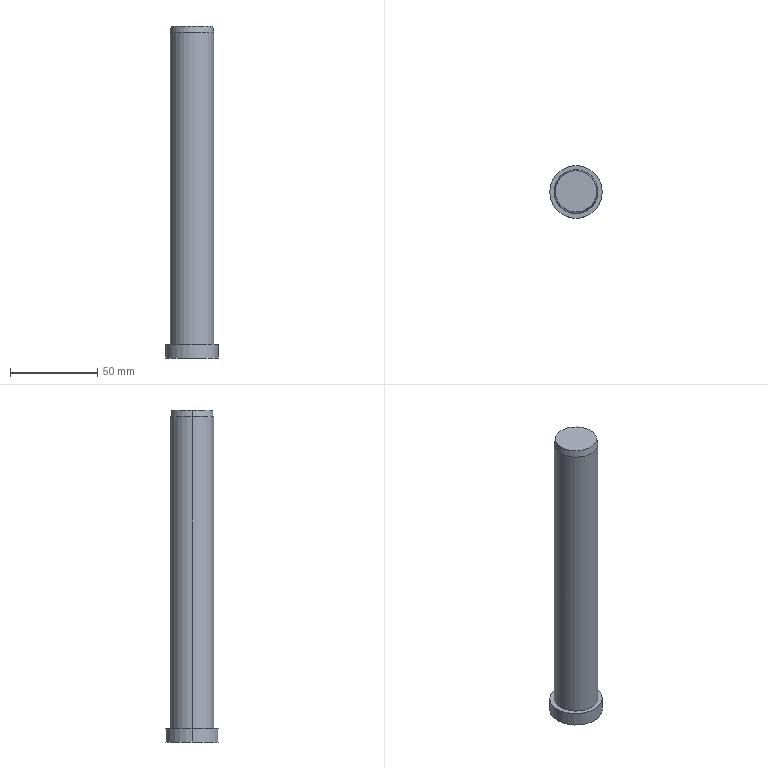Part | Creo | 1 solid | 15 faces | box 30 x 30 x 190 mm | volume 94190 mm3 | cylinder 8 | cone 4 | plane 3 | commonest cylinder face diameters 6.7 x2 25 x2 30 x2 7.98 x1 8 x1
STEP:
#1=CARTESIAN_POINT('',(0.,0.,0.));
#2=DIRECTION('',(0.,0.,1.));
#3=DIRECTION('',(1.,0.,0.));
#4=AXIS2_PLACEMENT_3D('',#1,#2,#3);
#5=CARTESIAN_POINT('',(-95.65,-141.,-276.5));
#6=VERTEX_POINT('',#5);
#7=CARTESIAN_POINT('',(-102.35,-141.,-276.5));
#8=VERTEX_POINT('',#7);
#9=CARTESIAN_POINT('',(-99.,-141.,-276.5));
#10=DIRECTION('',(0.,0.,-1.));
#11=DIRECTION('',(1.,0.,0.));
#12=AXIS2_PLACEMENT_3D('',#9,#10,#11);
#13=CIRCLE('',#12,3.35);
#14=EDGE_CURVE('',#6,#8,#13,.T.);
#15=ORIENTED_EDGE('',*,*,#14,.T.);
#16=CARTESIAN_POINT('',(-102.35,-141.,-295.5));
#17=VERTEX_POINT('',#16);
#18=CARTESIAN_POINT('',(-102.35,-141.,-295.5));
#19=DIRECTION('',(0.,0.,1.));
#20=VECTOR('',#19,19.);
#21=LINE('',#18,#20);
#22=EDGE_CURVE('',#17,#8,#21,.T.);
#23=ORIENTED_EDGE('',*,*,#22,.F.);
#24=CARTESIAN_POINT('',(-95.65,-141.,-295.5));
#25=VERTEX_POINT('',#24);
#26=CARTESIAN_POINT('',(-99.,-141.,-295.5));
#27=DIRECTION('',(0.,0.,1.));
#28=DIRECTION('',(-1.,0.,0.));
#29=AXIS2_PLACEMENT_3D('',#26,#27,#28);
#30=CIRCLE('',#29,3.35);
#31=EDGE_CURVE('',#17,#25,#30,.T.);
#32=ORIENTED_EDGE('',*,*,#31,.T.);
#33=CARTESIAN_POINT('',(-95.65,-141.,-295.5));
#34=DIRECTION('',(0.,0.,1.));
#35=VECTOR('',#34,19.);
#36=LINE('',#33,#35);
#37=EDGE_CURVE('',#25,#6,#36,.T.);
#38=ORIENTED_EDGE('',*,*,#37,.T.);
#39=EDGE_LOOP('',(#15,#23,#32,#38));
#40=FACE_OUTER_BOUND('',#39,.F.);
#41=CARTESIAN_POINT('',(-99.,-141.,-295.5));
#42=DIRECTION('',(0.,0.,1.));
#43=DIRECTION('',(1.,0.,0.));
#44=AXIS2_PLACEMENT_3D('',#41,#42,#43);
#45=CYLINDRICAL_SURFACE('',#44,3.35);
#46=ADVANCED_FACE('',(#40),#45,.F.);
#47=ORIENTED_EDGE('',*,*,#14,.F.);
#48=CARTESIAN_POINT('',(-99.,-141.,-274.487));
#49=VERTEX_POINT('',#48);
#50=CARTESIAN_POINT('',(-99.,-141.,-274.487));
#51=DIRECTION('',(0.8572,0.,-0.515));
#52=VECTOR('',#51,3.908);
#53=LINE('',#50,#52);
#54=EDGE_CURVE('',#49,#6,#53,.T.);
#55=ORIENTED_EDGE('',*,*,#54,.F.);
#56=CARTESIAN_POINT('',(-99.,-141.,-274.487));
#57=DIRECTION('',(-0.8572,0.,-0.515));
#58=VECTOR('',#57,3.908);
#59=LINE('',#56,#58);
#60=EDGE_CURVE('',#49,#8,#59,.T.);
#61=ORIENTED_EDGE('',*,*,#60,.T.);
#62=EDGE_LOOP('',(#47,#55,#61));
#63=FACE_OUTER_BOUND('',#62,.F.);
#64=CARTESIAN_POINT('',(-99.,-141.,-275.554));
#65=DIRECTION('',(0.,0.,-1.));
#66=DIRECTION('',(-1.,0.,0.));
#67=AXIS2_PLACEMENT_3D('',#64,#65,#66);
#68=CONICAL_SURFACE('',#67,1.775,59.);
#69=ADVANCED_FACE('',(#63),#68,.F.);
#70=CARTESIAN_POINT('',(-99.,-141.,-276.5));
#71=DIRECTION('',(0.,0.,-1.));
#72=DIRECTION('',(-1.,0.,0.));
#73=AXIS2_PLACEMENT_3D('',#70,#71,#72);
#74=CIRCLE('',#73,3.35);
#75=EDGE_CURVE('',#8,#6,#74,.T.);
#76=ORIENTED_EDGE('',*,*,#75,.F.);
#77=ORIENTED_EDGE('',*,*,#60,.F.);
#78=ORIENTED_EDGE('',*,*,#54,.T.);
#79=EDGE_LOOP('',(#76,#77,#78));
#80=FACE_OUTER_BOUND('',#79,.F.);
#81=CARTESIAN_POINT('',(-99.,-141.,-275.554));
#82=DIRECTION('',(0.,0.,-1.));
#83=DIRECTION('',(-1.,0.,0.));
#84=AXIS2_PLACEMENT_3D('',#81,#82,#83);
#85=CONICAL_SURFACE('',#84,1.775,59.);
#86=ADVANCED_FACE('',(#80),#85,.F.);
#87=ORIENTED_EDGE('',*,*,#75,.T.);
#88=ORIENTED_EDGE('',*,*,#37,.F.);
#89=CARTESIAN_POINT('',(-99.,-141.,-295.5));
#90=DIRECTION('',(0.,0.,1.));
#91=DIRECTION('',(1.,0.,0.));
#92=AXIS2_PLACEMENT_3D('',#89,#90,#91);
#93=CIRCLE('',#92,3.35);
#94=EDGE_CURVE('',#25,#17,#93,.T.);
#95=ORIENTED_EDGE('',*,*,#94,.T.);
#96=ORIENTED_EDGE('',*,*,#22,.T.);
#97=EDGE_LOOP('',(#87,#88,#95,#96));
#98=FACE_OUTER_BOUND('',#97,.F.);
#99=CARTESIAN_POINT('',(-99.,-141.,-295.5));
#100=DIRECTION('',(0.,0.,1.));
#101=DIRECTION('',(1.,0.,0.));
#102=AXIS2_PLACEMENT_3D('',#99,#100,#101);
#103=CYLINDRICAL_SURFACE('',#102,3.35);
#104=ADVANCED_FACE('',(#98),#103,.F.);
#105=CARTESIAN_POINT('',(-114.,-141.,-295.5));
#106=VERTEX_POINT('',#105);
#107=CARTESIAN_POINT('',(-84.,-141.,-295.5));
#108=VERTEX_POINT('',#107);
#109=CARTESIAN_POINT('',(-99.,-141.,-295.5));
#110=DIRECTION('',(0.,0.,-1.));
#111=DIRECTION('',(-1.,0.,0.));
#112=AXIS2_PLACEMENT_3D('',#109,#110,#111);
#113=CIRCLE('',#112,15.);
#114=EDGE_CURVE('',#106,#108,#113,.T.);
#115=ORIENTED_EDGE('',*,*,#114,.F.);
#116=CARTESIAN_POINT('',(-99.,-141.,-295.5));
#117=DIRECTION('',(0.,0.,-1.));
#118=DIRECTION('',(1.,0.,0.));
#119=AXIS2_PLACEMENT_3D('',#116,#117,#118);
#120=CIRCLE('',#119,15.);
#121=EDGE_CURVE('',#108,#106,#120,.T.);
#122=ORIENTED_EDGE('',*,*,#121,.F.);
#123=EDGE_LOOP('',(#115,#122));
#124=FACE_OUTER_BOUND('',#123,.F.);
#125=ORIENTED_EDGE('',*,*,#94,.F.);
#126=ORIENTED_EDGE('',*,*,#31,.F.);
#127=EDGE_LOOP('',(#125,#126));
#128=FACE_BOUND('',#127,.F.);
#129=CARTESIAN_POINT('',(-99.,-141.,-295.5));
#130=DIRECTION('',(0.,0.,-1.));
#131=DIRECTION('',(1.,0.,0.));
#132=AXIS2_PLACEMENT_3D('',#129,#130,#131);
#133=PLANE('',#132);
#134=ADVANCED_FACE('',(#124,#128),#133,.T.);
#135=CARTESIAN_POINT('',(-84.,-141.,-287.5));
#136=VERTEX_POINT('',#135);
#137=CARTESIAN_POINT('',(-114.,-141.,-287.5));
#138=VERTEX_POINT('',#137);
#139=CARTESIAN_POINT('',(-99.,-141.,-287.5));
#140=DIRECTION('',(0.,0.,1.));
#141=DIRECTION('',(1.,0.,0.));
#142=AXIS2_PLACEMENT_3D('',#139,#140,#141);
#143=CIRCLE('',#142,15.);
#144=EDGE_CURVE('',#136,#138,#143,.T.);
#145=ORIENTED_EDGE('',*,*,#144,.T.);
#146=CARTESIAN_POINT('',(-114.,-141.,-287.5));
#147=DIRECTION('',(0.,0.,-1.));
#148=VECTOR('',#147,8.);
#149=LINE('',#146,#148);
#150=EDGE_CURVE('',#138,#106,#149,.T.);
#151=ORIENTED_EDGE('',*,*,#150,.T.);
#152=ORIENTED_EDGE('',*,*,#114,.T.);
#153=CARTESIAN_POINT('',(-84.,-141.,-287.5));
#154=DIRECTION('',(0.,0.,-1.));
#155=VECTOR('',#154,8.);
#156=LINE('',#153,#155);
#157=EDGE_CURVE('',#136,#108,#156,.T.);
#158=ORIENTED_EDGE('',*,*,#157,.F.);
#159=EDGE_LOOP('',(#145,#151,#152,#158));
#160=FACE_OUTER_BOUND('',#159,.F.);
#161=CARTESIAN_POINT('',(-99.,-141.,-287.5));
#162=DIRECTION('',(0.,0.,-1.));
#163=DIRECTION('',(1.,0.,0.));
#164=AXIS2_PLACEMENT_3D('',#161,#162,#163);
#165=CYLINDRICAL_SURFACE('',#164,15.);
#166=ADVANCED_FACE('',(#160),#165,.T.);
#167=CARTESIAN_POINT('',(-99.,-141.,-287.5));
#168=DIRECTION('',(0.,0.,1.));
#169=DIRECTION('',(-1.,0.,0.));
#170=AXIS2_PLACEMENT_3D('',#167,#168,#169);
#171=CIRCLE('',#170,15.);
#172=EDGE_CURVE('',#138,#136,#171,.T.);
#173=ORIENTED_EDGE('',*,*,#172,.F.);
#174=ORIENTED_EDGE('',*,*,#144,.F.);
#175=EDGE_LOOP('',(#173,#174));
#176=FACE_OUTER_BOUND('',#175,.F.);
#177=CARTESIAN_POINT('',(-111.5,-141.,-287.5));
#178=VERTEX_POINT('',#177);
#179=CARTESIAN_POINT('',(-86.5,-141.,-287.5));
#180=VERTEX_POINT('',#179);
#181=CARTESIAN_POINT('',(-99.,-141.,-287.5));
#182=DIRECTION('',(0.,0.,-1.));
#183=DIRECTION('',(-1.,0.,0.));
#184=AXIS2_PLACEMENT_3D('',#181,#182,#183);
#185=CIRCLE('',#184,12.5);
#186=EDGE_CURVE('',#178,#180,#185,.T.);
#187=ORIENTED_EDGE('',*,*,#186,.F.);
#188=CARTESIAN_POINT('',(-99.,-141.,-287.5));
#189=DIRECTION('',(0.,0.,-1.));
#190=DIRECTION('',(1.,0.,0.));
#191=AXIS2_PLACEMENT_3D('',#188,#189,#190);
#192=CIRCLE('',#191,12.5);
#193=EDGE_CURVE('',#180,#178,#192,.T.);
#194=ORIENTED_EDGE('',*,*,#193,.F.);
#195=EDGE_LOOP('',(#187,#194));
#196=FACE_BOUND('',#195,.F.);
#197=CARTESIAN_POINT('',(-99.,-141.,-287.5));
#198=DIRECTION('',(0.,0.,-1.));
#199=DIRECTION('',(1.,0.,0.));
#200=AXIS2_PLACEMENT_3D('',#197,#198,#199);
#201=PLANE('',#200);
#202=ADVANCED_FACE('',(#176,#196),#201,.F.);
#203=CARTESIAN_POINT('',(-86.5,-141.,-109.5));
#204=VERTEX_POINT('',#203);
#205=CARTESIAN_POINT('',(-111.5,-141.,-109.5));
#206=VERTEX_POINT('',#205);
#207=CARTESIAN_POINT('',(-99.,-141.,-109.5));
#208=DIRECTION('',(0.,0.,1.));
#209=DIRECTION('',(1.,0.,0.));
#210=AXIS2_PLACEMENT_3D('',#207,#208,#209);
#211=CIRCLE('',#210,12.5);
#212=EDGE_CURVE('',#204,#206,#211,.T.);
#213=ORIENTED_EDGE('',*,*,#212,.T.);
#214=CARTESIAN_POINT('',(-111.5,-141.,-287.5));
#215=DIRECTION('',(0.,0.,1.));
#216=VECTOR('',#215,178.);
#217=LINE('',#214,#216);
#218=EDGE_CURVE('',#178,#206,#217,.T.);
#219=ORIENTED_EDGE('',*,*,#218,.F.);
#220=ORIENTED_EDGE('',*,*,#186,.T.);
#221=CARTESIAN_POINT('',(-86.5,-141.,-287.5));
#222=DIRECTION('',(0.,0.,1.));
#223=VECTOR('',#222,178.);
#224=LINE('',#221,#223);
#225=EDGE_CURVE('',#180,#204,#224,.T.);
#226=ORIENTED_EDGE('',*,*,#225,.T.);
#227=EDGE_LOOP('',(#213,#219,#220,#226));
#228=FACE_OUTER_BOUND('',#227,.F.);
#229=CARTESIAN_POINT('',(-99.,-141.,-287.5));
#230=DIRECTION('',(0.,0.,1.));
#231=DIRECTION('',(1.,0.,0.));
#232=AXIS2_PLACEMENT_3D('',#229,#230,#231);
#233=CYLINDRICAL_SURFACE('',#232,12.5);
#234=ADVANCED_FACE('',(#228),#233,.T.);
#235=ORIENTED_EDGE('',*,*,#212,.F.);
#236=CARTESIAN_POINT('',(-87.205,-141.,-105.5));
#237=VERTEX_POINT('',#236);
#238=CARTESIAN_POINT('',(-87.205,-141.,-105.5));
#239=DIRECTION('',(0.1736,0.,-0.9848));
#240=VECTOR('',#239,4.062);
#241=LINE('',#238,#240);
#242=EDGE_CURVE('',#237,#204,#241,.T.);
#243=ORIENTED_EDGE('',*,*,#242,.F.);
#244=CARTESIAN_POINT('',(-110.795,-141.,-105.5));
#245=VERTEX_POINT('',#244);
#246=CARTESIAN_POINT('',(-99.,-141.,-105.5));
#247=DIRECTION('',(0.,0.,1.));
#248=DIRECTION('',(1.,0.,0.));
#249=AXIS2_PLACEMENT_3D('',#246,#247,#248);
#250=CIRCLE('',#249,11.795);
#251=EDGE_CURVE('',#237,#245,#250,.T.);
#252=ORIENTED_EDGE('',*,*,#251,.T.);
#253=CARTESIAN_POINT('',(-110.795,-141.,-105.5));
#254=DIRECTION('',(-0.1736,0.,-0.9848));
#255=VECTOR('',#254,4.062);
#256=LINE('',#253,#255);
#257=EDGE_CURVE('',#245,#206,#256,.T.);
#258=ORIENTED_EDGE('',*,*,#257,.T.);
#259=EDGE_LOOP('',(#235,#243,#252,#258));
#260=FACE_OUTER_BOUND('',#259,.F.);
#261=CARTESIAN_POINT('',(-99.,-141.,-107.5));
#262=DIRECTION('',(0.,0.,-1.));
#263=DIRECTION('',(1.,0.,0.));
#264=AXIS2_PLACEMENT_3D('',#261,#262,#263);
#265=CONICAL_SURFACE('',#264,12.147,10.);
#266=ADVANCED_FACE('',(#260),#265,.T.);
#267=CARTESIAN_POINT('',(-99.,-141.,-109.5));
#268=DIRECTION('',(0.,0.,1.));
#269=DIRECTION('',(-1.,0.,0.));
#270=AXIS2_PLACEMENT_3D('',#267,#268,#269);
#271=CIRCLE('',#270,12.5);
#272=EDGE_CURVE('',#206,#204,#271,.T.);
#273=ORIENTED_EDGE('',*,*,#272,.F.);
#274=ORIENTED_EDGE('',*,*,#257,.F.);
#275=CARTESIAN_POINT('',(-99.,-141.,-105.5));
#276=DIRECTION('',(0.,0.,1.));
#277=DIRECTION('',(-1.,0.,0.));
#278=AXIS2_PLACEMENT_3D('',#275,#276,#277);
#279=CIRCLE('',#278,11.795);
#280=EDGE_CURVE('',#245,#237,#279,.T.);
#281=ORIENTED_EDGE('',*,*,#280,.T.);
#282=ORIENTED_EDGE('',*,*,#242,.T.);
#283=EDGE_LOOP('',(#273,#274,#281,#282));
#284=FACE_OUTER_BOUND('',#283,.F.);
#285=CARTESIAN_POINT('',(-99.,-141.,-107.5));
#286=DIRECTION('',(0.,0.,-1.));
#287=DIRECTION('',(1.,0.,0.));
#288=AXIS2_PLACEMENT_3D('',#285,#286,#287);
#289=CONICAL_SURFACE('',#288,12.147,10.);
#290=ADVANCED_FACE('',(#284),#289,.T.);
#291=ORIENTED_EDGE('',*,*,#272,.T.);
#292=ORIENTED_EDGE('',*,*,#225,.F.);
#293=ORIENTED_EDGE('',*,*,#193,.T.);
#294=ORIENTED_EDGE('',*,*,#218,.T.);
#295=EDGE_LOOP('',(#291,#292,#293,#294));
#296=FACE_OUTER_BOUND('',#295,.F.);
#297=CARTESIAN_POINT('',(-99.,-141.,-287.5));
#298=DIRECTION('',(0.,0.,1.));
#299=DIRECTION('',(1.,0.,0.));
#300=AXIS2_PLACEMENT_3D('',#297,#298,#299);
#301=CYLINDRICAL_SURFACE('',#300,12.5);
#302=ADVANCED_FACE('',(#296),#301,.T.);
#303=ORIENTED_EDGE('',*,*,#251,.F.);
#304=ORIENTED_EDGE('',*,*,#280,.F.);
#305=EDGE_LOOP('',(#303,#304));
#306=FACE_OUTER_BOUND('',#305,.F.);
#307=CARTESIAN_POINT('',(-99.,-141.,-105.5));
#308=DIRECTION('',(0.,0.,1.));
#309=DIRECTION('',(1.,0.,0.));
#310=AXIS2_PLACEMENT_3D('',#307,#308,#309);
#311=PLANE('',#310);
#312=ADVANCED_FACE('',(#306),#311,.T.);
#313=ORIENTED_EDGE('',*,*,#172,.T.);
#314=ORIENTED_EDGE('',*,*,#157,.T.);
#315=ORIENTED_EDGE('',*,*,#121,.T.);
#316=ORIENTED_EDGE('',*,*,#150,.F.);
#317=EDGE_LOOP('',(#313,#314,#315,#316));
#318=FACE_OUTER_BOUND('',#317,.F.);
#319=CARTESIAN_POINT('',(-99.,-141.,-287.5));
#320=DIRECTION('',(0.,0.,-1.));
#321=DIRECTION('',(1.,0.,0.));
#322=AXIS2_PLACEMENT_3D('',#319,#320,#321);
#323=CYLINDRICAL_SURFACE('',#322,15.);
#324=ADVANCED_FACE('',(#318),#323,.T.);
#325=CLOSED_SHELL('',(#46,#69,#86,#104,#134,#166,#202,#234,#266,#290,#302,#312,#324));
#326=CARTESIAN_POINT('',(-95.005,-141.,-295.5));
#327=VERTEX_POINT('',#326);
#328=CARTESIAN_POINT('',(-102.99,-141.,-295.5));
#329=VERTEX_POINT('',#328);
#330=CARTESIAN_POINT('',(-99.,-141.,-295.5));
#331=DIRECTION('',(0.,0.,1.));
#332=DIRECTION('',(1.,0.,0.));
#333=AXIS2_PLACEMENT_3D('',#330,#331,#332);
#334=CIRCLE('',#333,3.99);
#335=EDGE_CURVE('',#327,#329,#334,.T.);
#336=ORIENTED_EDGE('',*,*,#335,.F.);
#337=CARTESIAN_POINT('',(-95.01,-141.,-279.5));
#338=VERTEX_POINT('',#337);
#339=CARTESIAN_POINT('',(-95.005,-141.,-295.5));
#340=DIRECTION('',(0.,0.,1.));
#341=VECTOR('',#340,16.);
#342=LINE('',#339,#341);
#343=EDGE_CURVE('',#327,#338,#342,.T.);
#344=ORIENTED_EDGE('',*,*,#343,.T.);
#345=CARTESIAN_POINT('',(-102.99,-141.,-279.5));
#346=VERTEX_POINT('',#345);
#347=CARTESIAN_POINT('',(-99.,-141.,-279.5));
#348=DIRECTION('',(0.,0.,-1.));
#349=DIRECTION('',(-1.,0.,0.));
#350=AXIS2_PLACEMENT_3D('',#347,#348,#349);
#351=CIRCLE('',#350,3.99);
#352=EDGE_CURVE('',#346,#338,#351,.T.);
#353=ORIENTED_EDGE('',*,*,#352,.F.);
#354=CARTESIAN_POINT('',(-99.,-144.99,-279.5));
#355=VERTEX_POINT('',#354);
#356=CARTESIAN_POINT('',(-99.,-141.,-279.5));
#357=DIRECTION('',(0.,0.,-1.));
#358=DIRECTION('',(0.,-1.,0.));
#359=AXIS2_PLACEMENT_3D('',#356,#357,#358);
#360=CIRCLE('',#359,3.99);
#361=EDGE_CURVE('',#355,#346,#360,.T.);
#362=ORIENTED_EDGE('',*,*,#361,.F.);
#363=CARTESIAN_POINT('',(-99.,-144.995,-295.5));
#364=VERTEX_POINT('',#363);
#365=CARTESIAN_POINT('',(-99.,-144.995,-279.5));
#366=DIRECTION('',(0.,0.,-1.));
#367=VECTOR('',#366,16.);
#368=LINE('',#365,#367);
#369=EDGE_CURVE('',#355,#364,#368,.T.);
#370=ORIENTED_EDGE('',*,*,#369,.T.);
#371=CARTESIAN_POINT('',(-99.,-141.,-295.5));
#372=DIRECTION('',(0.,0.,1.));
#373=DIRECTION('',(-1.,-0.000002843,0.));
#374=AXIS2_PLACEMENT_3D('',#371,#372,#373);
#375=CIRCLE('',#374,3.99);
#376=EDGE_CURVE('',#329,#364,#375,.T.);
#377=ORIENTED_EDGE('',*,*,#376,.F.);
#378=EDGE_LOOP('',(#336,#344,#353,#362,#370,#377));
#379=FACE_OUTER_BOUND('',#378,.F.);
#380=CARTESIAN_POINT('',(-99.,-141.,-296.5));
#381=DIRECTION('',(0.,0.,1.));
#382=DIRECTION('',(1.,0.,0.));
#383=AXIS2_PLACEMENT_3D('',#380,#381,#382);
#384=CYLINDRICAL_SURFACE('',#383,4.);
#385=ADVANCED_FACE('',(#379),#384,.T.);
#386=ORIENTED_EDGE('',*,*,#335,.T.);
#387=ORIENTED_EDGE('',*,*,#376,.T.);
#388=ORIENTED_EDGE('',*,*,#369,.F.);
#389=ORIENTED_EDGE('',*,*,#361,.T.);
#390=ORIENTED_EDGE('',*,*,#352,.T.);
#391=ORIENTED_EDGE('',*,*,#343,.F.);
#392=EDGE_LOOP('',(#386,#387,#388,#389,#390,#391));
#393=FACE_OUTER_BOUND('',#392,.F.);
#394=CARTESIAN_POINT('',(-99.,-141.,-295.5));
#395=DIRECTION('',(0.,0.,1.));
#396=DIRECTION('',(1.,0.,0.));
#397=AXIS2_PLACEMENT_3D('',#394,#395,#396);
#398=CYLINDRICAL_SURFACE('',#397,3.99);
#399=ADVANCED_FACE('',(#393),#398,.F.);
#400=CLOSED_SHELL('',(#385,#399));
#401=ORIENTED_CLOSED_SHELL('',*,#400,.F.);
#402=BREP_WITH_VOIDS('',#325,(#401));
#403=(LENGTH_UNIT()NAMED_UNIT(*)SI_UNIT(.MILLI.,.METRE.));
#404=UNCERTAINTY_MEASURE_WITH_UNIT(LENGTH_MEASURE(0.01947),#403,'','');
#405=(NAMED_UNIT(*)PLANE_ANGLE_UNIT()SI_UNIT($,.RADIAN.));
#406=PLANE_ANGLE_MEASURE_WITH_UNIT(PLANE_ANGLE_MEASURE(0.01745),#405);
#407=(CONVERSION_BASED_UNIT('DEGREE',#406)NAMED_UNIT(*)PLANE_ANGLE_UNIT());
#408=(NAMED_UNIT(*)SI_UNIT($,.STERADIAN.)SOLID_ANGLE_UNIT());
#409=(GEOMETRIC_REPRESENTATION_CONTEXT(3)GLOBAL_UNCERTAINTY_ASSIGNED_CONTEXT((#404))GLOBAL_UNIT_ASSIGNED_CONTEXT((#403,#407,#408))REPRESENTATION_CONTEXT('',''));
#410=ADVANCED_BREP_SHAPE_REPRESENTATION('',(#4,#402),#409);